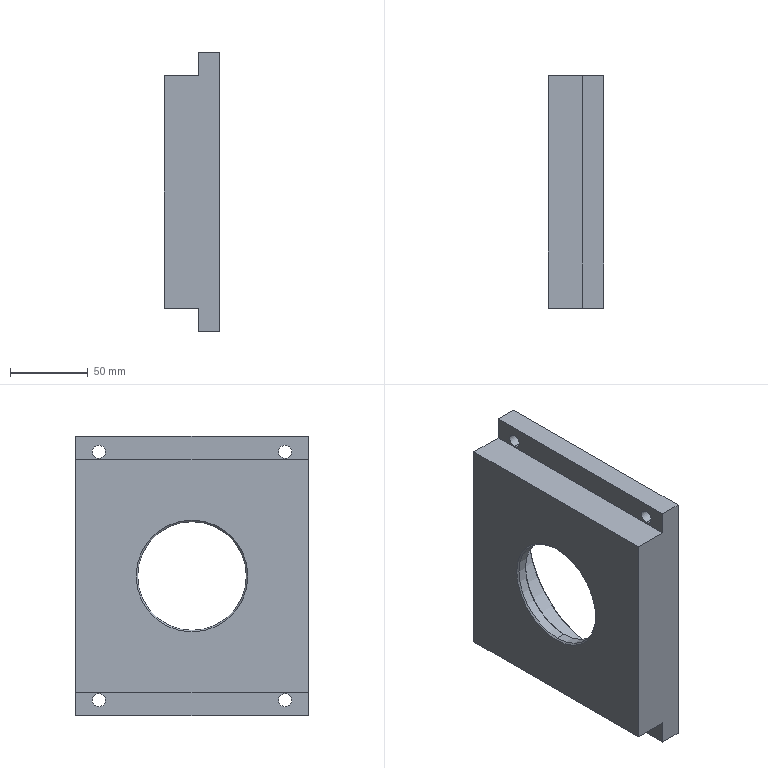Part | SolidWorks | features BaseBody 1 | 1 solid | 42 faces | box 36 x 150 x 180 mm | volume 519040 mm3 | cylinder 18 | cone 12 | plane 12 | commonest cylinder face diameters 8.5 x8 30.5 x4 70 x2 110 x2 120 x2
STEP:
#1=CARTESIAN_POINT('',(17.,0.,60.));
#2=VERTEX_POINT('',#1);
#3=CARTESIAN_POINT('',(17.,0.,-60.));
#4=VERTEX_POINT('',#3);
#5=CARTESIAN_POINT('',(17.,0.,0.));
#6=DIRECTION('',(1.,0.,0.));
#7=DIRECTION('',(0.,0.,-1.));
#8=AXIS2_PLACEMENT_3D('',#5,#6,#7);
#9=CIRCLE('',#8,60.);
#10=EDGE_CURVE('',#2,#4,#9,.T.);
#11=ORIENTED_EDGE('',*,*,#10,.F.);
#12=CARTESIAN_POINT('',(18.,0.,61.));
#13=VERTEX_POINT('',#12);
#14=CARTESIAN_POINT('',(17.,0.,60.));
#15=DIRECTION('',(0.7071,0.,0.7071));
#16=VECTOR('',#15,1000.);
#17=LINE('',#14,#16);
#18=EDGE_CURVE('',#2,#13,#17,.T.);
#19=ORIENTED_EDGE('',*,*,#18,.T.);
#20=CARTESIAN_POINT('',(18.,0.,-61.));
#21=VERTEX_POINT('',#20);
#22=CARTESIAN_POINT('',(18.,0.,0.));
#23=DIRECTION('',(-1.,0.,0.));
#24=DIRECTION('',(0.,0.,-1.));
#25=AXIS2_PLACEMENT_3D('',#22,#23,#24);
#26=CIRCLE('',#25,61.);
#27=EDGE_CURVE('',#21,#13,#26,.T.);
#28=ORIENTED_EDGE('',*,*,#27,.F.);
#29=CARTESIAN_POINT('',(17.,0.,-60.));
#30=DIRECTION('',(0.7071,0.,-0.7071));
#31=VECTOR('',#30,1000.);
#32=LINE('',#29,#31);
#33=EDGE_CURVE('',#4,#21,#32,.T.);
#34=ORIENTED_EDGE('',*,*,#33,.F.);
#35=EDGE_LOOP('',(#11,#19,#28,#34));
#36=FACE_OUTER_BOUND('',#35,.T.);
#37=CARTESIAN_POINT('',(17.,0.,0.));
#38=DIRECTION('',(1.,0.,0.));
#39=DIRECTION('',(0.,0.,-1.));
#40=AXIS2_PLACEMENT_3D('',#37,#38,#39);
#41=CONICAL_SURFACE('',#40,60.,0.7854);
#42=ADVANCED_FACE('',(#36),#41,.F.);
#43=CARTESIAN_POINT('',(-11.,0.,35.));
#44=VERTEX_POINT('',#43);
#45=CARTESIAN_POINT('',(-11.,0.,-35.));
#46=VERTEX_POINT('',#45);
#47=CARTESIAN_POINT('',(-11.,0.,0.));
#48=DIRECTION('',(1.,0.,0.));
#49=DIRECTION('',(0.,0.,-1.));
#50=AXIS2_PLACEMENT_3D('',#47,#48,#49);
#51=CIRCLE('',#50,35.);
#52=EDGE_CURVE('',#44,#46,#51,.T.);
#53=ORIENTED_EDGE('',*,*,#52,.F.);
#54=CARTESIAN_POINT('',(-10.,0.,36.));
#55=VERTEX_POINT('',#54);
#56=CARTESIAN_POINT('',(-11.,0.,35.));
#57=DIRECTION('',(0.7071,0.,0.7071));
#58=VECTOR('',#57,1000.);
#59=LINE('',#56,#58);
#60=EDGE_CURVE('',#44,#55,#59,.T.);
#61=ORIENTED_EDGE('',*,*,#60,.T.);
#62=CARTESIAN_POINT('',(-10.,0.,-36.));
#63=VERTEX_POINT('',#62);
#64=CARTESIAN_POINT('',(-10.,0.,0.));
#65=DIRECTION('',(-1.,0.,0.));
#66=DIRECTION('',(0.,0.,-1.));
#67=AXIS2_PLACEMENT_3D('',#64,#65,#66);
#68=CIRCLE('',#67,36.);
#69=EDGE_CURVE('',#63,#55,#68,.T.);
#70=ORIENTED_EDGE('',*,*,#69,.F.);
#71=CARTESIAN_POINT('',(-11.,0.,-35.));
#72=DIRECTION('',(0.7071,0.,-0.7071));
#73=VECTOR('',#72,1000.);
#74=LINE('',#71,#73);
#75=EDGE_CURVE('',#46,#63,#74,.T.);
#76=ORIENTED_EDGE('',*,*,#75,.F.);
#77=EDGE_LOOP('',(#53,#61,#70,#76));
#78=FACE_OUTER_BOUND('',#77,.T.);
#79=CARTESIAN_POINT('',(-11.,0.,0.));
#80=DIRECTION('',(1.,0.,0.));
#81=DIRECTION('',(0.,0.,-1.));
#82=AXIS2_PLACEMENT_3D('',#79,#80,#81);
#83=CONICAL_SURFACE('',#82,35.,0.7854);
#84=ADVANCED_FACE('',(#78),#83,.F.);
#85=CARTESIAN_POINT('',(-17.,0.,-35.));
#86=VERTEX_POINT('',#85);
#87=CARTESIAN_POINT('',(-17.,0.,35.));
#88=VERTEX_POINT('',#87);
#89=CARTESIAN_POINT('',(-17.,0.,0.));
#90=DIRECTION('',(-1.,0.,0.));
#91=DIRECTION('',(0.,0.,-1.));
#92=AXIS2_PLACEMENT_3D('',#89,#90,#91);
#93=CIRCLE('',#92,35.);
#94=EDGE_CURVE('',#86,#88,#93,.T.);
#95=ORIENTED_EDGE('',*,*,#94,.F.);
#96=CARTESIAN_POINT('',(-18.,0.,-36.));
#97=VERTEX_POINT('',#96);
#98=CARTESIAN_POINT('',(-18.,0.,-36.));
#99=DIRECTION('',(-0.7071,0.,-0.7071));
#100=VECTOR('',#99,1000.);
#101=LINE('',#98,#100);
#102=EDGE_CURVE('',#86,#97,#101,.T.);
#103=ORIENTED_EDGE('',*,*,#102,.T.);
#104=CARTESIAN_POINT('',(-18.,0.,36.));
#105=VERTEX_POINT('',#104);
#106=CARTESIAN_POINT('',(-18.,0.,0.));
#107=DIRECTION('',(1.,0.,0.));
#108=DIRECTION('',(0.,0.,-1.));
#109=AXIS2_PLACEMENT_3D('',#106,#107,#108);
#110=CIRCLE('',#109,36.);
#111=EDGE_CURVE('',#105,#97,#110,.T.);
#112=ORIENTED_EDGE('',*,*,#111,.F.);
#113=CARTESIAN_POINT('',(-18.,0.,36.));
#114=DIRECTION('',(-0.7071,0.,0.7071));
#115=VECTOR('',#114,1000.);
#116=LINE('',#113,#115);
#117=EDGE_CURVE('',#88,#105,#116,.T.);
#118=ORIENTED_EDGE('',*,*,#117,.F.);
#119=EDGE_LOOP('',(#95,#103,#112,#118));
#120=FACE_OUTER_BOUND('',#119,.T.);
#121=CARTESIAN_POINT('',(-18.,0.,0.));
#122=DIRECTION('',(-1.,0.,0.));
#123=DIRECTION('',(0.,0.,1.));
#124=AXIS2_PLACEMENT_3D('',#121,#122,#123);
#125=CONICAL_SURFACE('',#124,36.,0.7854);
#126=ADVANCED_FACE('',(#120),#125,.F.);
#127=CARTESIAN_POINT('',(-6.,0.,55.));
#128=VERTEX_POINT('',#127);
#129=CARTESIAN_POINT('',(-6.,0.,-55.));
#130=VERTEX_POINT('',#129);
#131=CARTESIAN_POINT('',(-6.,0.,0.));
#132=DIRECTION('',(1.,0.,0.));
#133=DIRECTION('',(0.,0.,-1.));
#134=AXIS2_PLACEMENT_3D('',#131,#132,#133);
#135=CIRCLE('',#134,55.);
#136=EDGE_CURVE('',#128,#130,#135,.T.);
#137=ORIENTED_EDGE('',*,*,#136,.F.);
#138=CARTESIAN_POINT('',(-5.,0.,56.));
#139=VERTEX_POINT('',#138);
#140=CARTESIAN_POINT('',(-6.,0.,55.));
#141=DIRECTION('',(0.7071,0.,0.7071));
#142=VECTOR('',#141,1000.);
#143=LINE('',#140,#142);
#144=EDGE_CURVE('',#128,#139,#143,.T.);
#145=ORIENTED_EDGE('',*,*,#144,.T.);
#146=CARTESIAN_POINT('',(-5.,0.,-56.));
#147=VERTEX_POINT('',#146);
#148=CARTESIAN_POINT('',(-5.,0.,0.));
#149=DIRECTION('',(-1.,0.,0.));
#150=DIRECTION('',(0.,0.,-1.));
#151=AXIS2_PLACEMENT_3D('',#148,#149,#150);
#152=CIRCLE('',#151,56.);
#153=EDGE_CURVE('',#147,#139,#152,.T.);
#154=ORIENTED_EDGE('',*,*,#153,.F.);
#155=CARTESIAN_POINT('',(-6.,0.,-55.));
#156=DIRECTION('',(0.7071,0.,-0.7071));
#157=VECTOR('',#156,1000.);
#158=LINE('',#155,#157);
#159=EDGE_CURVE('',#130,#147,#158,.T.);
#160=ORIENTED_EDGE('',*,*,#159,.F.);
#161=EDGE_LOOP('',(#137,#145,#154,#160));
#162=FACE_OUTER_BOUND('',#161,.T.);
#163=CARTESIAN_POINT('',(-6.,0.,0.));
#164=DIRECTION('',(1.,0.,0.));
#165=DIRECTION('',(0.,0.,-1.));
#166=AXIS2_PLACEMENT_3D('',#163,#164,#165);
#167=CONICAL_SURFACE('',#166,55.,0.7854);
#168=ADVANCED_FACE('',(#162),#167,.F.);
#169=CARTESIAN_POINT('',(0.,70.,-60.25));
#170=VERTEX_POINT('',#169);
#171=CARTESIAN_POINT('',(0.,70.,-29.75));
#172=VERTEX_POINT('',#171);
#173=CARTESIAN_POINT('',(0.,70.,-45.));
#174=DIRECTION('',(0.,1.,0.));
#175=DIRECTION('',(0.,0.,1.));
#176=AXIS2_PLACEMENT_3D('',#173,#174,#175);
#177=CIRCLE('',#176,15.25);
#178=EDGE_CURVE('',#170,#172,#177,.T.);
#179=ORIENTED_EDGE('',*,*,#178,.F.);
#180=CARTESIAN_POINT('',(0.,75.,-60.25));
#181=VERTEX_POINT('',#180);
#182=CARTESIAN_POINT('',(0.,75.,-60.25));
#183=DIRECTION('',(0.,1.,0.));
#184=VECTOR('',#183,1000.);
#185=LINE('',#182,#184);
#186=EDGE_CURVE('',#170,#181,#185,.T.);
#187=ORIENTED_EDGE('',*,*,#186,.T.);
#188=CARTESIAN_POINT('',(0.,75.,-29.75));
#189=VERTEX_POINT('',#188);
#190=CARTESIAN_POINT('',(0.,75.,-45.));
#191=DIRECTION('',(0.,1.,0.));
#192=DIRECTION('',(0.,0.,1.));
#193=AXIS2_PLACEMENT_3D('',#190,#191,#192);
#194=CIRCLE('',#193,15.25);
#195=EDGE_CURVE('',#181,#189,#194,.T.);
#196=ORIENTED_EDGE('',*,*,#195,.T.);
#197=CARTESIAN_POINT('',(0.,75.,-29.75));
#198=DIRECTION('',(0.,1.,0.));
#199=VECTOR('',#198,1000.);
#200=LINE('',#197,#199);
#201=EDGE_CURVE('',#172,#189,#200,.T.);
#202=ORIENTED_EDGE('',*,*,#201,.F.);
#203=EDGE_LOOP('',(#179,#187,#196,#202));
#204=FACE_OUTER_BOUND('',#203,.T.);
#205=CARTESIAN_POINT('',(0.,75.,-45.));
#206=DIRECTION('',(0.,1.,0.));
#207=DIRECTION('',(0.,0.,1.));
#208=AXIS2_PLACEMENT_3D('',#205,#206,#207);
#209=CYLINDRICAL_SURFACE('',#208,15.25);
#210=ADVANCED_FACE('',(#204),#209,.F.);
#211=CARTESIAN_POINT('',(0.,60.837,-45.));
#212=VERTEX_POINT('',#211);
#213=CARTESIAN_POINT('',(0.,70.,-29.75));
#214=DIRECTION('',(0.,0.515,0.8572));
#215=VECTOR('',#214,1000.);
#216=LINE('',#213,#215);
#217=EDGE_CURVE('',#212,#172,#216,.T.);
#218=ORIENTED_EDGE('',*,*,#217,.F.);
#219=CARTESIAN_POINT('',(0.,70.,-60.25));
#220=DIRECTION('',(0.,0.515,-0.8572));
#221=VECTOR('',#220,1000.);
#222=LINE('',#219,#221);
#223=EDGE_CURVE('',#212,#170,#222,.T.);
#224=ORIENTED_EDGE('',*,*,#223,.T.);
#225=ORIENTED_EDGE('',*,*,#178,.T.);
#226=EDGE_LOOP('',(#218,#224,#225));
#227=FACE_OUTER_BOUND('',#226,.T.);
#228=CARTESIAN_POINT('',(0.,70.,-45.));
#229=DIRECTION('',(0.,1.,0.));
#230=DIRECTION('',(0.,0.,1.));
#231=AXIS2_PLACEMENT_3D('',#228,#229,#230);
#232=CONICAL_SURFACE('',#231,15.25,1.03);
#233=ADVANCED_FACE('',(#227),#232,.F.);
#234=CARTESIAN_POINT('',(0.,70.,29.75));
#235=VERTEX_POINT('',#234);
#236=CARTESIAN_POINT('',(0.,70.,60.25));
#237=VERTEX_POINT('',#236);
#238=CARTESIAN_POINT('',(0.,70.,45.));
#239=DIRECTION('',(0.,1.,0.));
#240=DIRECTION('',(0.,0.,1.));
#241=AXIS2_PLACEMENT_3D('',#238,#239,#240);
#242=CIRCLE('',#241,15.25);
#243=EDGE_CURVE('',#235,#237,#242,.T.);
#244=ORIENTED_EDGE('',*,*,#243,.F.);
#245=CARTESIAN_POINT('',(0.,75.,29.75));
#246=VERTEX_POINT('',#245);
#247=CARTESIAN_POINT('',(0.,75.,29.75));
#248=DIRECTION('',(0.,1.,0.));
#249=VECTOR('',#248,1000.);
#250=LINE('',#247,#249);
#251=EDGE_CURVE('',#235,#246,#250,.T.);
#252=ORIENTED_EDGE('',*,*,#251,.T.);
#253=CARTESIAN_POINT('',(0.,75.,60.25));
#254=VERTEX_POINT('',#253);
#255=CARTESIAN_POINT('',(0.,75.,45.));
#256=DIRECTION('',(0.,1.,0.));
#257=DIRECTION('',(0.,0.,1.));
#258=AXIS2_PLACEMENT_3D('',#255,#256,#257);
#259=CIRCLE('',#258,15.25);
#260=EDGE_CURVE('',#246,#254,#259,.T.);
#261=ORIENTED_EDGE('',*,*,#260,.T.);
#262=CARTESIAN_POINT('',(0.,75.,60.25));
#263=DIRECTION('',(0.,1.,0.));
#264=VECTOR('',#263,1000.);
#265=LINE('',#262,#264);
#266=EDGE_CURVE('',#237,#254,#265,.T.);
#267=ORIENTED_EDGE('',*,*,#266,.F.);
#268=EDGE_LOOP('',(#244,#252,#261,#267));
#269=FACE_OUTER_BOUND('',#268,.T.);
#270=CARTESIAN_POINT('',(0.,75.,45.));
#271=DIRECTION('',(0.,1.,0.));
#272=DIRECTION('',(0.,0.,1.));
#273=AXIS2_PLACEMENT_3D('',#270,#271,#272);
#274=CYLINDRICAL_SURFACE('',#273,15.25);
#275=ADVANCED_FACE('',(#269),#274,.F.);
#276=CARTESIAN_POINT('',(0.,60.837,45.));
#277=VERTEX_POINT('',#276);
#278=CARTESIAN_POINT('',(0.,70.,60.25));
#279=DIRECTION('',(0.,0.515,0.8572));
#280=VECTOR('',#279,1000.);
#281=LINE('',#278,#280);
#282=EDGE_CURVE('',#277,#237,#281,.T.);
#283=ORIENTED_EDGE('',*,*,#282,.F.);
#284=CARTESIAN_POINT('',(0.,70.,29.75));
#285=DIRECTION('',(0.,0.515,-0.8572));
#286=VECTOR('',#285,1000.);
#287=LINE('',#284,#286);
#288=EDGE_CURVE('',#277,#235,#287,.T.);
#289=ORIENTED_EDGE('',*,*,#288,.T.);
#290=ORIENTED_EDGE('',*,*,#243,.T.);
#291=EDGE_LOOP('',(#283,#289,#290));
#292=FACE_OUTER_BOUND('',#291,.T.);
#293=CARTESIAN_POINT('',(0.,70.,45.));
#294=DIRECTION('',(0.,1.,0.));
#295=DIRECTION('',(0.,0.,1.));
#296=AXIS2_PLACEMENT_3D('',#293,#294,#295);
#297=CONICAL_SURFACE('',#296,15.25,1.03);
#298=ADVANCED_FACE('',(#292),#297,.F.);
#299=CARTESIAN_POINT('',(4.,60.,84.25));
#300=VERTEX_POINT('',#299);
#301=CARTESIAN_POINT('',(4.,60.,75.75));
#302=VERTEX_POINT('',#301);
#303=CARTESIAN_POINT('',(4.,60.,80.));
#304=DIRECTION('',(1.,0.,0.));
#305=DIRECTION('',(0.,0.,-1.));
#306=AXIS2_PLACEMENT_3D('',#303,#304,#305);
#307=CIRCLE('',#306,4.25);
#308=EDGE_CURVE('',#300,#302,#307,.T.);
#309=ORIENTED_EDGE('',*,*,#308,.F.);
#310=CARTESIAN_POINT('',(18.,60.,84.25));
#311=VERTEX_POINT('',#310);
#312=CARTESIAN_POINT('',(18.,60.,84.25));
#313=DIRECTION('',(1.,0.,0.));
#314=VECTOR('',#313,1000.);
#315=LINE('',#312,#314);
#316=EDGE_CURVE('',#300,#311,#315,.T.);
#317=ORIENTED_EDGE('',*,*,#316,.T.);
#318=CARTESIAN_POINT('',(18.,60.,75.75));
#319=VERTEX_POINT('',#318);
#320=CARTESIAN_POINT('',(18.,60.,80.));
#321=DIRECTION('',(1.,0.,0.));
#322=DIRECTION('',(0.,0.,-1.));
#323=AXIS2_PLACEMENT_3D('',#320,#321,#322);
#324=CIRCLE('',#323,4.25);
#325=EDGE_CURVE('',#311,#319,#324,.T.);
#326=ORIENTED_EDGE('',*,*,#325,.T.);
#327=CARTESIAN_POINT('',(18.,60.,75.75));
#328=DIRECTION('',(1.,0.,0.));
#329=VECTOR('',#328,1000.);
#330=LINE('',#327,#329);
#331=EDGE_CURVE('',#302,#319,#330,.T.);
#332=ORIENTED_EDGE('',*,*,#331,.F.);
#333=EDGE_LOOP('',(#309,#317,#326,#332));
#334=FACE_OUTER_BOUND('',#333,.T.);
#335=CARTESIAN_POINT('',(18.,60.,80.));
#336=DIRECTION('',(1.,0.,0.));
#337=DIRECTION('',(0.,0.,-1.));
#338=AXIS2_PLACEMENT_3D('',#335,#336,#337);
#339=CYLINDRICAL_SURFACE('',#338,4.25);
#340=ADVANCED_FACE('',(#334),#339,.F.);
#341=CARTESIAN_POINT('',(4.,60.,-75.75));
#342=VERTEX_POINT('',#341);
#343=CARTESIAN_POINT('',(4.,60.,-84.25));
#344=VERTEX_POINT('',#343);
#345=CARTESIAN_POINT('',(4.,60.,-80.));
#346=DIRECTION('',(1.,0.,0.));
#347=DIRECTION('',(0.,0.,-1.));
#348=AXIS2_PLACEMENT_3D('',#345,#346,#347);
#349=CIRCLE('',#348,4.25);
#350=EDGE_CURVE('',#342,#344,#349,.T.);
#351=ORIENTED_EDGE('',*,*,#350,.F.);
#352=CARTESIAN_POINT('',(18.,60.,-75.75));
#353=VERTEX_POINT('',#352);
#354=CARTESIAN_POINT('',(18.,60.,-75.75));
#355=DIRECTION('',(1.,0.,0.));
#356=VECTOR('',#355,1000.);
#357=LINE('',#354,#356);
#358=EDGE_CURVE('',#342,#353,#357,.T.);
#359=ORIENTED_EDGE('',*,*,#358,.T.);
#360=CARTESIAN_POINT('',(18.,60.,-84.25));
#361=VERTEX_POINT('',#360);
#362=CARTESIAN_POINT('',(18.,60.,-80.));
#363=DIRECTION('',(1.,0.,0.));
#364=DIRECTION('',(0.,0.,-1.));
#365=AXIS2_PLACEMENT_3D('',#362,#363,#364);
#366=CIRCLE('',#365,4.25);
#367=EDGE_CURVE('',#353,#361,#366,.T.);
#368=ORIENTED_EDGE('',*,*,#367,.T.);
#369=CARTESIAN_POINT('',(18.,60.,-84.25));
#370=DIRECTION('',(1.,0.,0.));
#371=VECTOR('',#370,1000.);
#372=LINE('',#369,#371);
#373=EDGE_CURVE('',#344,#361,#372,.T.);
#374=ORIENTED_EDGE('',*,*,#373,.F.);
#375=EDGE_LOOP('',(#351,#359,#368,#374));
#376=FACE_OUTER_BOUND('',#375,.T.);
#377=CARTESIAN_POINT('',(18.,60.,-80.));
#378=DIRECTION('',(1.,0.,0.));
#379=DIRECTION('',(0.,0.,-1.));
#380=AXIS2_PLACEMENT_3D('',#377,#378,#379);
#381=CYLINDRICAL_SURFACE('',#380,4.25);
#382=ADVANCED_FACE('',(#376),#381,.F.);
#383=CARTESIAN_POINT('',(4.,-60.,-75.75));
#384=VERTEX_POINT('',#383);
#385=CARTESIAN_POINT('',(4.,-60.,-84.25));
#386=VERTEX_POINT('',#385);
#387=CARTESIAN_POINT('',(4.,-60.,-80.));
#388=DIRECTION('',(1.,0.,0.));
#389=DIRECTION('',(0.,0.,-1.));
#390=AXIS2_PLACEMENT_3D('',#387,#388,#389);
#391=CIRCLE('',#390,4.25);
#392=EDGE_CURVE('',#384,#386,#391,.T.);
#393=ORIENTED_EDGE('',*,*,#392,.F.);
#394=CARTESIAN_POINT('',(18.,-60.,-75.75));
#395=VERTEX_POINT('',#394);
#396=CARTESIAN_POINT('',(18.,-60.,-75.75));
#397=DIRECTION('',(1.,0.,0.));
#398=VECTOR('',#397,1000.);
#399=LINE('',#396,#398);
#400=EDGE_CURVE('',#384,#395,#399,.T.);
#401=ORIENTED_EDGE('',*,*,#400,.T.);
#402=CARTESIAN_POINT('',(18.,-60.,-84.25));
#403=VERTEX_POINT('',#402);
#404=CARTESIAN_POINT('',(18.,-60.,-80.));
#405=DIRECTION('',(1.,0.,0.));
#406=DIRECTION('',(0.,0.,-1.));
#407=AXIS2_PLACEMENT_3D('',#404,#405,#406);
#408=CIRCLE('',#407,4.25);
#409=EDGE_CURVE('',#395,#403,#408,.T.);
#410=ORIENTED_EDGE('',*,*,#409,.T.);
#411=CARTESIAN_POINT('',(18.,-60.,-84.25));
#412=DIRECTION('',(1.,0.,0.));
#413=VECTOR('',#412,1000.);
#414=LINE('',#411,#413);
#415=EDGE_CURVE('',#386,#403,#414,.T.);
#416=ORIENTED_EDGE('',*,*,#415,.F.);
#417=EDGE_LOOP('',(#393,#401,#410,#416));
#418=FACE_OUTER_BOUND('',#417,.T.);
#419=CARTESIAN_POINT('',(18.,-60.,-80.));
#420=DIRECTION('',(1.,0.,0.));
#421=DIRECTION('',(0.,0.,-1.));
#422=AXIS2_PLACEMENT_3D('',#419,#420,#421);
#423=CYLINDRICAL_SURFACE('',#422,4.25);
#424=ADVANCED_FACE('',(#418),#423,.F.);
#425=CARTESIAN_POINT('',(4.,-60.,84.25));
#426=VERTEX_POINT('',#425);
#427=CARTESIAN_POINT('',(4.,-60.,75.75));
#428=VERTEX_POINT('',#427);
#429=CARTESIAN_POINT('',(4.,-60.,80.));
#430=DIRECTION('',(1.,0.,0.));
#431=DIRECTION('',(0.,0.,-1.));
#432=AXIS2_PLACEMENT_3D('',#429,#430,#431);
#433=CIRCLE('',#432,4.25);
#434=EDGE_CURVE('',#426,#428,#433,.T.);
#435=ORIENTED_EDGE('',*,*,#434,.F.);
#436=CARTESIAN_POINT('',(18.,-60.,84.25));
#437=VERTEX_POINT('',#436);
#438=CARTESIAN_POINT('',(18.,-60.,84.25));
#439=DIRECTION('',(1.,0.,0.));
#440=VECTOR('',#439,1000.);
#441=LINE('',#438,#440);
#442=EDGE_CURVE('',#426,#437,#441,.T.);
#443=ORIENTED_EDGE('',*,*,#442,.T.);
#444=CARTESIAN_POINT('',(18.,-60.,75.75));
#445=VERTEX_POINT('',#444);
#446=CARTESIAN_POINT('',(18.,-60.,80.));
#447=DIRECTION('',(1.,0.,0.));
#448=DIRECTION('',(0.,0.,-1.));
#449=AXIS2_PLACEMENT_3D('',#446,#447,#448);
#450=CIRCLE('',#449,4.25);
#451=EDGE_CURVE('',#437,#445,#450,.T.);
#452=ORIENTED_EDGE('',*,*,#451,.T.);
#453=CARTESIAN_POINT('',(18.,-60.,75.75));
#454=DIRECTION('',(1.,0.,0.));
#455=VECTOR('',#454,1000.);
#456=LINE('',#453,#455);
#457=EDGE_CURVE('',#428,#445,#456,.T.);
#458=ORIENTED_EDGE('',*,*,#457,.F.);
#459=EDGE_LOOP('',(#435,#443,#452,#458));
#460=FACE_OUTER_BOUND('',#459,.T.);
#461=CARTESIAN_POINT('',(18.,-60.,80.));
#462=DIRECTION('',(1.,0.,0.));
#463=DIRECTION('',(0.,0.,-1.));
#464=AXIS2_PLACEMENT_3D('',#461,#462,#463);
#465=CYLINDRICAL_SURFACE('',#464,4.25);
#466=ADVANCED_FACE('',(#460),#465,.F.);
#467=CARTESIAN_POINT('',(-10.,0.,55.));
#468=VERTEX_POINT('',#467);
#469=CARTESIAN_POINT('',(-10.,0.,-55.));
#470=VERTEX_POINT('',#469);
#471=CARTESIAN_POINT('',(-10.,0.,0.));
#472=DIRECTION('',(1.,0.,0.));
#473=DIRECTION('',(0.,0.,-1.));
#474=AXIS2_PLACEMENT_3D('',#471,#472,#473);
#475=CIRCLE('',#474,55.);
#476=EDGE_CURVE('',#468,#470,#475,.T.);
#477=ORIENTED_EDGE('',*,*,#476,.F.);
#478=CARTESIAN_POINT('',(-10.,0.,55.));
#479=DIRECTION('',(1.,0.,0.));
#480=VECTOR('',#479,1000.);
#481=LINE('',#478,#480);
#482=EDGE_CURVE('',#468,#128,#481,.T.);
#483=ORIENTED_EDGE('',*,*,#482,.T.);
#484=ORIENTED_EDGE('',*,*,#136,.T.);
#485=CARTESIAN_POINT('',(-10.,0.,-55.));
#486=DIRECTION('',(1.,0.,0.));
#487=VECTOR('',#486,1000.);
#488=LINE('',#485,#487);
#489=EDGE_CURVE('',#470,#130,#488,.T.);
#490=ORIENTED_EDGE('',*,*,#489,.F.);
#491=EDGE_LOOP('',(#477,#483,#484,#490));
#492=FACE_OUTER_BOUND('',#491,.T.);
#493=CARTESIAN_POINT('',(-10.,0.,0.));
#494=DIRECTION('',(1.,0.,0.));
#495=DIRECTION('',(0.,0.,-1.));
#496=AXIS2_PLACEMENT_3D('',#493,#494,#495);
#497=CYLINDRICAL_SURFACE('',#496,55.);
#498=ADVANCED_FACE('',(#492),#497,.F.);
#499=CARTESIAN_POINT('',(-5.,0.,60.));
#500=VERTEX_POINT('',#499);
#501=CARTESIAN_POINT('',(-5.,0.,-60.));
#502=VERTEX_POINT('',#501);
#503=CARTESIAN_POINT('',(-5.,0.,0.));
#504=DIRECTION('',(1.,0.,0.));
#505=DIRECTION('',(0.,0.,-1.));
#506=AXIS2_PLACEMENT_3D('',#503,#504,#505);
#507=CIRCLE('',#506,60.);
#508=EDGE_CURVE('',#500,#502,#507,.T.);
#509=ORIENTED_EDGE('',*,*,#508,.F.);
#510=CARTESIAN_POINT('',(-5.,0.,60.));
#511=DIRECTION('',(1.,0.,0.));
#512=VECTOR('',#511,1000.);
#513=LINE('',#510,#512);
#514=EDGE_CURVE('',#500,#2,#513,.T.);
#515=ORIENTED_EDGE('',*,*,#514,.T.);
#516=ORIENTED_EDGE('',*,*,#10,.T.);
#517=CARTESIAN_POINT('',(-5.,0.,-60.));
#518=DIRECTION('',(1.,0.,0.));
#519=VECTOR('',#518,1000.);
#520=LINE('',#517,#519);
#521=EDGE_CURVE('',#502,#4,#520,.T.);
#522=ORIENTED_EDGE('',*,*,#521,.F.);
#523=EDGE_LOOP('',(#509,#515,#516,#522));
#524=FACE_OUTER_BOUND('',#523,.T.);
#525=CARTESIAN_POINT('',(-5.,0.,0.));
#526=DIRECTION('',(1.,0.,0.));
#527=DIRECTION('',(0.,0.,-1.));
#528=AXIS2_PLACEMENT_3D('',#525,#526,#527);
#529=CYLINDRICAL_SURFACE('',#528,60.);
#530=ADVANCED_FACE('',(#524),#529,.F.);
#531=ORIENTED_EDGE('',*,*,#52,.T.);
#532=CARTESIAN_POINT('',(18.,0.,-35.));
#533=DIRECTION('',(-1.,0.,0.));
#534=VECTOR('',#533,1000.);
#535=LINE('',#532,#534);
#536=EDGE_CURVE('',#46,#86,#535,.T.);
#537=ORIENTED_EDGE('',*,*,#536,.T.);
#538=ORIENTED_EDGE('',*,*,#94,.T.);
#539=CARTESIAN_POINT('',(18.,0.,35.));
#540=DIRECTION('',(-1.,0.,0.));
#541=VECTOR('',#540,1000.);
#542=LINE('',#539,#541);
#543=EDGE_CURVE('',#44,#88,#542,.T.);
#544=ORIENTED_EDGE('',*,*,#543,.F.);
#545=EDGE_LOOP('',(#531,#537,#538,#544));
#546=FACE_OUTER_BOUND('',#545,.T.);
#547=CARTESIAN_POINT('',(18.,0.,0.));
#548=DIRECTION('',(-1.,0.,0.));
#549=DIRECTION('',(0.,0.,1.));
#550=AXIS2_PLACEMENT_3D('',#547,#548,#549);
#551=CYLINDRICAL_SURFACE('',#550,35.);
#552=ADVANCED_FACE('',(#546),#551,.F.);
#553=ORIENTED_EDGE('',*,*,#536,.F.);
#554=CARTESIAN_POINT('',(-11.,0.,0.));
#555=DIRECTION('',(1.,0.,0.));
#556=DIRECTION('',(0.,0.,-1.));
#557=AXIS2_PLACEMENT_3D('',#554,#555,#556);
#558=CIRCLE('',#557,35.);
#559=EDGE_CURVE('',#46,#44,#558,.T.);
#560=ORIENTED_EDGE('',*,*,#559,.T.);
#561=ORIENTED_EDGE('',*,*,#543,.T.);
#562=CARTESIAN_POINT('',(-17.,0.,0.));
#563=DIRECTION('',(-1.,0.,0.));
#564=DIRECTION('',(0.,0.,-1.));
#565=AXIS2_PLACEMENT_3D('',#562,#563,#564);
#566=CIRCLE('',#565,35.);
#567=EDGE_CURVE('',#88,#86,#566,.T.);
#568=ORIENTED_EDGE('',*,*,#567,.T.);
#569=EDGE_LOOP('',(#553,#560,#561,#568));
#570=FACE_OUTER_BOUND('',#569,.T.);
#571=CARTESIAN_POINT('',(18.,0.,0.));
#572=DIRECTION('',(-1.,0.,0.));
#573=DIRECTION('',(0.,0.,1.));
#574=AXIS2_PLACEMENT_3D('',#571,#572,#573);
#575=CYLINDRICAL_SURFACE('',#574,35.);
#576=ADVANCED_FACE('',(#570),#575,.F.);
#577=ORIENTED_EDGE('',*,*,#27,.T.);
#578=CARTESIAN_POINT('',(18.,0.,0.));
#579=DIRECTION('',(-1.,0.,0.));
#580=DIRECTION('',(0.,0.,-1.));
#581=AXIS2_PLACEMENT_3D('',#578,#579,#580);
#582=CIRCLE('',#581,61.);
#583=EDGE_CURVE('',#13,#21,#582,.T.);
#584=ORIENTED_EDGE('',*,*,#583,.T.);
#585=EDGE_LOOP('',(#577,#584));
#586=FACE_BOUND('',#585,.T.);
#587=CARTESIAN_POINT('',(18.,60.,80.));
#588=DIRECTION('',(1.,0.,0.));
#589=DIRECTION('',(0.,0.,-1.));
#590=AXIS2_PLACEMENT_3D('',#587,#588,#589);
#591=CIRCLE('',#590,4.25);
#592=EDGE_CURVE('',#319,#311,#591,.T.);
#593=ORIENTED_EDGE('',*,*,#592,.F.);
#594=ORIENTED_EDGE('',*,*,#325,.F.);
#595=EDGE_LOOP('',(#593,#594));
#596=FACE_BOUND('',#595,.T.);
#597=CARTESIAN_POINT('',(18.,60.,-80.));
#598=DIRECTION('',(1.,0.,0.));
#599=DIRECTION('',(0.,0.,-1.));
#600=AXIS2_PLACEMENT_3D('',#597,#598,#599);
#601=CIRCLE('',#600,4.25);
#602=EDGE_CURVE('',#361,#353,#601,.T.);
#603=ORIENTED_EDGE('',*,*,#602,.F.);
#604=ORIENTED_EDGE('',*,*,#367,.F.);
#605=EDGE_LOOP('',(#603,#604));
#606=FACE_BOUND('',#605,.T.);
#607=CARTESIAN_POINT('',(18.,-60.,-80.));
#608=DIRECTION('',(1.,0.,0.));
#609=DIRECTION('',(0.,0.,-1.));
#610=AXIS2_PLACEMENT_3D('',#607,#608,#609);
#611=CIRCLE('',#610,4.25);
#612=EDGE_CURVE('',#403,#395,#611,.T.);
#613=ORIENTED_EDGE('',*,*,#612,.F.);
#614=ORIENTED_EDGE('',*,*,#409,.F.);
#615=EDGE_LOOP('',(#613,#614));
#616=FACE_BOUND('',#615,.T.);
#617=CARTESIAN_POINT('',(18.,-60.,80.));
#618=DIRECTION('',(1.,0.,0.));
#619=DIRECTION('',(0.,0.,-1.));
#620=AXIS2_PLACEMENT_3D('',#617,#618,#619);
#621=CIRCLE('',#620,4.25);
#622=EDGE_CURVE('',#445,#437,#621,.T.);
#623=ORIENTED_EDGE('',*,*,#622,.F.);
#624=ORIENTED_EDGE('',*,*,#451,.F.);
#625=EDGE_LOOP('',(#623,#624));
#626=FACE_BOUND('',#625,.T.);
#627=CARTESIAN_POINT('',(18.,-75.,-90.));
#628=VERTEX_POINT('',#627);
#629=CARTESIAN_POINT('',(18.,75.,-90.));
#630=VERTEX_POINT('',#629);
#631=CARTESIAN_POINT('',(18.,75.,-90.));
#632=DIRECTION('',(0.,1.,0.));
#633=VECTOR('',#632,1000.);
#634=LINE('',#631,#633);
#635=EDGE_CURVE('',#628,#630,#634,.T.);
#636=ORIENTED_EDGE('',*,*,#635,.T.);
#637=CARTESIAN_POINT('',(18.,75.,90.));
#638=VERTEX_POINT('',#637);
#639=CARTESIAN_POINT('',(18.,75.,90.));
#640=DIRECTION('',(0.,0.,1.));
#641=VECTOR('',#640,1000.);
#642=LINE('',#639,#641);
#643=EDGE_CURVE('',#630,#638,#642,.T.);
#644=ORIENTED_EDGE('',*,*,#643,.T.);
#645=CARTESIAN_POINT('',(18.,-75.,90.));
#646=VERTEX_POINT('',#645);
#647=CARTESIAN_POINT('',(18.,75.,90.));
#648=DIRECTION('',(0.,-1.,0.));
#649=VECTOR('',#648,1000.);
#650=LINE('',#647,#649);
#651=EDGE_CURVE('',#638,#646,#650,.T.);
#652=ORIENTED_EDGE('',*,*,#651,.T.);
#653=CARTESIAN_POINT('',(18.,-75.,90.));
#654=DIRECTION('',(0.,0.,-1.));
#655=VECTOR('',#654,1000.);
#656=LINE('',#653,#655);
#657=EDGE_CURVE('',#646,#628,#656,.T.);
#658=ORIENTED_EDGE('',*,*,#657,.T.);
#659=EDGE_LOOP('',(#636,#644,#652,#658));
#660=FACE_OUTER_BOUND('',#659,.T.);
#661=CARTESIAN_POINT('',(18.,0.,0.));
#662=DIRECTION('',(1.,0.,0.));
#663=DIRECTION('',(0.,0.,-1.));
#664=AXIS2_PLACEMENT_3D('',#661,#662,#663);
#665=PLANE('',#664);
#666=ADVANCED_FACE('',(#586,#596,#606,#616,#626,#660),#665,.T.);
#667=ORIENTED_EDGE('',*,*,#111,.T.);
#668=CARTESIAN_POINT('',(-18.,0.,0.));
#669=DIRECTION('',(1.,0.,0.));
#670=DIRECTION('',(0.,0.,-1.));
#671=AXIS2_PLACEMENT_3D('',#668,#669,#670);
#672=CIRCLE('',#671,36.);
#673=EDGE_CURVE('',#97,#105,#672,.T.);
#674=ORIENTED_EDGE('',*,*,#673,.T.);
#675=EDGE_LOOP('',(#667,#674));
#676=FACE_BOUND('',#675,.T.);
#677=CARTESIAN_POINT('',(-18.,75.,-75.));
#678=VERTEX_POINT('',#677);
#679=CARTESIAN_POINT('',(-18.,75.,75.));
#680=VERTEX_POINT('',#679);
#681=CARTESIAN_POINT('',(-18.,75.,90.));
#682=DIRECTION('',(0.,0.,1.));
#683=VECTOR('',#682,1000.);
#684=LINE('',#681,#683);
#685=EDGE_CURVE('',#678,#680,#684,.T.);
#686=ORIENTED_EDGE('',*,*,#685,.F.);
#687=CARTESIAN_POINT('',(-18.,-75.,-75.));
#688=VERTEX_POINT('',#687);
#689=CARTESIAN_POINT('',(-18.,-75.,-75.));
#690=DIRECTION('',(0.,1.,0.));
#691=VECTOR('',#690,1000.);
#692=LINE('',#689,#691);
#693=EDGE_CURVE('',#688,#678,#692,.T.);
#694=ORIENTED_EDGE('',*,*,#693,.F.);
#695=CARTESIAN_POINT('',(-18.,-75.,75.));
#696=VERTEX_POINT('',#695);
#697=CARTESIAN_POINT('',(-18.,-75.,90.));
#698=DIRECTION('',(0.,0.,-1.));
#699=VECTOR('',#698,1000.);
#700=LINE('',#697,#699);
#701=EDGE_CURVE('',#696,#688,#700,.T.);
#702=ORIENTED_EDGE('',*,*,#701,.F.);
#703=CARTESIAN_POINT('',(-18.,-75.,75.));
#704=DIRECTION('',(0.,1.,0.));
#705=VECTOR('',#704,1000.);
#706=LINE('',#703,#705);
#707=EDGE_CURVE('',#696,#680,#706,.T.);
#708=ORIENTED_EDGE('',*,*,#707,.T.);
#709=EDGE_LOOP('',(#686,#694,#702,#708));
#710=FACE_OUTER_BOUND('',#709,.T.);
#711=CARTESIAN_POINT('',(-18.,0.,0.));
#712=DIRECTION('',(1.,0.,0.));
#713=DIRECTION('',(0.,0.,-1.));
#714=AXIS2_PLACEMENT_3D('',#711,#712,#713);
#715=PLANE('',#714);
#716=ADVANCED_FACE('',(#676,#710),#715,.F.);
#717=CARTESIAN_POINT('',(4.,-75.,-90.));
#718=VERTEX_POINT('',#717);
#719=CARTESIAN_POINT('',(18.,-75.,-90.));
#720=DIRECTION('',(-1.,0.,0.));
#721=VECTOR('',#720,1000.);
#722=LINE('',#719,#721);
#723=EDGE_CURVE('',#628,#718,#722,.T.);
#724=ORIENTED_EDGE('',*,*,#723,.T.);
#725=CARTESIAN_POINT('',(4.,75.,-90.));
#726=VERTEX_POINT('',#725);
#727=CARTESIAN_POINT('',(4.,-75.,-90.));
#728=DIRECTION('',(0.,1.,0.));
#729=VECTOR('',#728,1000.);
#730=LINE('',#727,#729);
#731=EDGE_CURVE('',#718,#726,#730,.T.);
#732=ORIENTED_EDGE('',*,*,#731,.T.);
#733=CARTESIAN_POINT('',(18.,75.,-90.));
#734=DIRECTION('',(-1.,0.,0.));
#735=VECTOR('',#734,1000.);
#736=LINE('',#733,#735);
#737=EDGE_CURVE('',#630,#726,#736,.T.);
#738=ORIENTED_EDGE('',*,*,#737,.F.);
#739=ORIENTED_EDGE('',*,*,#635,.F.);
#740=EDGE_LOOP('',(#724,#732,#738,#739));
#741=FACE_OUTER_BOUND('',#740,.T.);
#742=CARTESIAN_POINT('',(18.,75.,-90.));
#743=DIRECTION('',(0.,0.,1.));
#744=DIRECTION('',(1.,0.,0.));
#745=AXIS2_PLACEMENT_3D('',#742,#743,#744);
#746=PLANE('',#745);
#747=ADVANCED_FACE('',(#741),#746,.F.);
#748=CARTESIAN_POINT('',(0.,75.,-45.));
#749=DIRECTION('',(0.,1.,0.));
#750=DIRECTION('',(0.,0.,1.));
#751=AXIS2_PLACEMENT_3D('',#748,#749,#750);
#752=CIRCLE('',#751,15.25);
#753=EDGE_CURVE('',#189,#181,#752,.T.);
#754=ORIENTED_EDGE('',*,*,#753,.F.);
#755=ORIENTED_EDGE('',*,*,#195,.F.);
#756=EDGE_LOOP('',(#754,#755));
#757=FACE_BOUND('',#756,.T.);
#758=CARTESIAN_POINT('',(0.,75.,45.));
#759=DIRECTION('',(0.,1.,0.));
#760=DIRECTION('',(0.,0.,1.));
#761=AXIS2_PLACEMENT_3D('',#758,#759,#760);
#762=CIRCLE('',#761,15.25);
#763=EDGE_CURVE('',#254,#246,#762,.T.);
#764=ORIENTED_EDGE('',*,*,#763,.F.);
#765=ORIENTED_EDGE('',*,*,#260,.F.);
#766=EDGE_LOOP('',(#764,#765));
#767=FACE_BOUND('',#766,.T.);
#768=ORIENTED_EDGE('',*,*,#737,.T.);
#769=CARTESIAN_POINT('',(4.,75.,-75.));
#770=VERTEX_POINT('',#769);
#771=CARTESIAN_POINT('',(4.,75.,-90.));
#772=DIRECTION('',(0.,0.,-1.));
#773=VECTOR('',#772,1000.);
#774=LINE('',#771,#773);
#775=EDGE_CURVE('',#770,#726,#774,.T.);
#776=ORIENTED_EDGE('',*,*,#775,.F.);
#777=CARTESIAN_POINT('',(-18.,75.,-75.));
#778=DIRECTION('',(1.,0.,0.));
#779=VECTOR('',#778,1000.);
#780=LINE('',#777,#779);
#781=EDGE_CURVE('',#678,#770,#780,.T.);
#782=ORIENTED_EDGE('',*,*,#781,.F.);
#783=ORIENTED_EDGE('',*,*,#685,.T.);
#784=CARTESIAN_POINT('',(4.,75.,75.));
#785=VERTEX_POINT('',#784);
#786=CARTESIAN_POINT('',(-18.,75.,75.));
#787=DIRECTION('',(-1.,0.,0.));
#788=VECTOR('',#787,1000.);
#789=LINE('',#786,#788);
#790=EDGE_CURVE('',#785,#680,#789,.T.);
#791=ORIENTED_EDGE('',*,*,#790,.F.);
#792=CARTESIAN_POINT('',(4.,75.,90.));
#793=VERTEX_POINT('',#792);
#794=CARTESIAN_POINT('',(4.,75.,90.));
#795=DIRECTION('',(0.,0.,-1.));
#796=VECTOR('',#795,1000.);
#797=LINE('',#794,#796);
#798=EDGE_CURVE('',#793,#785,#797,.T.);
#799=ORIENTED_EDGE('',*,*,#798,.F.);
#800=CARTESIAN_POINT('',(18.,75.,90.));
#801=DIRECTION('',(-1.,0.,0.));
#802=VECTOR('',#801,1000.);
#803=LINE('',#800,#802);
#804=EDGE_CURVE('',#638,#793,#803,.T.);
#805=ORIENTED_EDGE('',*,*,#804,.F.);
#806=ORIENTED_EDGE('',*,*,#643,.F.);
#807=EDGE_LOOP('',(#768,#776,#782,#783,#791,#799,#805,#806));
#808=FACE_OUTER_BOUND('',#807,.T.);
#809=CARTESIAN_POINT('',(18.,75.,90.));
#810=DIRECTION('',(0.,-1.,0.));
#811=DIRECTION('',(0.,0.,-1.));
#812=AXIS2_PLACEMENT_3D('',#809,#810,#811);
#813=PLANE('',#812);
#814=ADVANCED_FACE('',(#757,#767,#808),#813,.F.);
#815=ORIENTED_EDGE('',*,*,#804,.T.);
#816=CARTESIAN_POINT('',(4.,-75.,90.));
#817=VERTEX_POINT('',#816);
#818=CARTESIAN_POINT('',(4.,-75.,90.));
#819=DIRECTION('',(0.,1.,0.));
#820=VECTOR('',#819,1000.);
#821=LINE('',#818,#820);
#822=EDGE_CURVE('',#817,#793,#821,.T.);
#823=ORIENTED_EDGE('',*,*,#822,.F.);
#824=CARTESIAN_POINT('',(18.,-75.,90.));
#825=DIRECTION('',(-1.,0.,0.));
#826=VECTOR('',#825,1000.);
#827=LINE('',#824,#826);
#828=EDGE_CURVE('',#646,#817,#827,.T.);
#829=ORIENTED_EDGE('',*,*,#828,.F.);
#830=ORIENTED_EDGE('',*,*,#651,.F.);
#831=EDGE_LOOP('',(#815,#823,#829,#830));
#832=FACE_OUTER_BOUND('',#831,.T.);
#833=CARTESIAN_POINT('',(18.,75.,90.));
#834=DIRECTION('',(0.,0.,-1.));
#835=DIRECTION('',(-1.,0.,0.));
#836=AXIS2_PLACEMENT_3D('',#833,#834,#835);
#837=PLANE('',#836);
#838=ADVANCED_FACE('',(#832),#837,.F.);
#839=CARTESIAN_POINT('',(4.,-75.,-75.));
#840=VERTEX_POINT('',#839);
#841=CARTESIAN_POINT('',(-18.,-75.,-75.));
#842=DIRECTION('',(1.,0.,0.));
#843=VECTOR('',#842,1000.);
#844=LINE('',#841,#843);
#845=EDGE_CURVE('',#688,#840,#844,.T.);
#846=ORIENTED_EDGE('',*,*,#845,.T.);
#847=CARTESIAN_POINT('',(4.,-75.,-90.));
#848=DIRECTION('',(0.,0.,-1.));
#849=VECTOR('',#848,1000.);
#850=LINE('',#847,#849);
#851=EDGE_CURVE('',#840,#718,#850,.T.);
#852=ORIENTED_EDGE('',*,*,#851,.T.);
#853=ORIENTED_EDGE('',*,*,#723,.F.);
#854=ORIENTED_EDGE('',*,*,#657,.F.);
#855=ORIENTED_EDGE('',*,*,#828,.T.);
#856=CARTESIAN_POINT('',(4.,-75.,75.));
#857=VERTEX_POINT('',#856);
#858=CARTESIAN_POINT('',(4.,-75.,90.));
#859=DIRECTION('',(0.,0.,-1.));
#860=VECTOR('',#859,1000.);
#861=LINE('',#858,#860);
#862=EDGE_CURVE('',#817,#857,#861,.T.);
#863=ORIENTED_EDGE('',*,*,#862,.T.);
#864=CARTESIAN_POINT('',(-18.,-75.,75.));
#865=DIRECTION('',(-1.,0.,0.));
#866=VECTOR('',#865,1000.);
#867=LINE('',#864,#866);
#868=EDGE_CURVE('',#857,#696,#867,.T.);
#869=ORIENTED_EDGE('',*,*,#868,.T.);
#870=ORIENTED_EDGE('',*,*,#701,.T.);
#871=EDGE_LOOP('',(#846,#852,#853,#854,#855,#863,#869,#870));
#872=FACE_OUTER_BOUND('',#871,.T.);
#873=CARTESIAN_POINT('',(18.,-75.,90.));
#874=DIRECTION('',(0.,1.,0.));
#875=DIRECTION('',(0.,0.,1.));
#876=AXIS2_PLACEMENT_3D('',#873,#874,#875);
#877=PLANE('',#876);
#878=ADVANCED_FACE('',(#872),#877,.F.);
#879=ORIENTED_EDGE('',*,*,#514,.F.);
#880=CARTESIAN_POINT('',(-5.,0.,0.));
#881=DIRECTION('',(1.,0.,0.));
#882=DIRECTION('',(0.,0.,-1.));
#883=AXIS2_PLACEMENT_3D('',#880,#881,#882);
#884=CIRCLE('',#883,60.);
#885=EDGE_CURVE('',#502,#500,#884,.T.);
#886=ORIENTED_EDGE('',*,*,#885,.F.);
#887=ORIENTED_EDGE('',*,*,#521,.T.);
#888=CARTESIAN_POINT('',(17.,0.,0.));
#889=DIRECTION('',(1.,0.,0.));
#890=DIRECTION('',(0.,0.,-1.));
#891=AXIS2_PLACEMENT_3D('',#888,#889,#890);
#892=CIRCLE('',#891,60.);
#893=EDGE_CURVE('',#4,#2,#892,.T.);
#894=ORIENTED_EDGE('',*,*,#893,.T.);
#895=EDGE_LOOP('',(#879,#886,#887,#894));
#896=FACE_OUTER_BOUND('',#895,.T.);
#897=CARTESIAN_POINT('',(-5.,0.,0.));
#898=DIRECTION('',(1.,0.,0.));
#899=DIRECTION('',(0.,0.,-1.));
#900=AXIS2_PLACEMENT_3D('',#897,#898,#899);
#901=CYLINDRICAL_SURFACE('',#900,60.);
#902=ADVANCED_FACE('',(#896),#901,.F.);
#903=ORIENTED_EDGE('',*,*,#153,.T.);
#904=CARTESIAN_POINT('',(-5.,0.,0.));
#905=DIRECTION('',(-1.,0.,0.));
#906=DIRECTION('',(0.,0.,-1.));
#907=AXIS2_PLACEMENT_3D('',#904,#905,#906);
#908=CIRCLE('',#907,56.);
#909=EDGE_CURVE('',#139,#147,#908,.T.);
#910=ORIENTED_EDGE('',*,*,#909,.T.);
#911=EDGE_LOOP('',(#903,#910));
#912=FACE_BOUND('',#911,.T.);
#913=ORIENTED_EDGE('',*,*,#885,.T.);
#914=ORIENTED_EDGE('',*,*,#508,.T.);
#915=EDGE_LOOP('',(#913,#914));
#916=FACE_OUTER_BOUND('',#915,.T.);
#917=CARTESIAN_POINT('',(-5.,0.,0.));
#918=DIRECTION('',(1.,0.,0.));
#919=DIRECTION('',(0.,0.,-1.));
#920=AXIS2_PLACEMENT_3D('',#917,#918,#919);
#921=PLANE('',#920);
#922=ADVANCED_FACE('',(#912,#916),#921,.T.);
#923=ORIENTED_EDGE('',*,*,#482,.F.);
#924=CARTESIAN_POINT('',(-10.,0.,0.));
#925=DIRECTION('',(1.,0.,0.));
#926=DIRECTION('',(0.,0.,-1.));
#927=AXIS2_PLACEMENT_3D('',#924,#925,#926);
#928=CIRCLE('',#927,55.);
#929=EDGE_CURVE('',#470,#468,#928,.T.);
#930=ORIENTED_EDGE('',*,*,#929,.F.);
#931=ORIENTED_EDGE('',*,*,#489,.T.);
#932=CARTESIAN_POINT('',(-6.,0.,0.));
#933=DIRECTION('',(1.,0.,0.));
#934=DIRECTION('',(0.,0.,-1.));
#935=AXIS2_PLACEMENT_3D('',#932,#933,#934);
#936=CIRCLE('',#935,55.);
#937=EDGE_CURVE('',#130,#128,#936,.T.);
#938=ORIENTED_EDGE('',*,*,#937,.T.);
#939=EDGE_LOOP('',(#923,#930,#931,#938));
#940=FACE_OUTER_BOUND('',#939,.T.);
#941=CARTESIAN_POINT('',(-10.,0.,0.));
#942=DIRECTION('',(1.,0.,0.));
#943=DIRECTION('',(0.,0.,-1.));
#944=AXIS2_PLACEMENT_3D('',#941,#942,#943);
#945=CYLINDRICAL_SURFACE('',#944,55.);
#946=ADVANCED_FACE('',(#940),#945,.F.);
#947=ORIENTED_EDGE('',*,*,#69,.T.);
#948=CARTESIAN_POINT('',(-10.,0.,0.));
#949=DIRECTION('',(-1.,0.,0.));
#950=DIRECTION('',(0.,0.,-1.));
#951=AXIS2_PLACEMENT_3D('',#948,#949,#950);
#952=CIRCLE('',#951,36.);
#953=EDGE_CURVE('',#55,#63,#952,.T.);
#954=ORIENTED_EDGE('',*,*,#953,.T.);
#955=EDGE_LOOP('',(#947,#954));
#956=FACE_BOUND('',#955,.T.);
#957=ORIENTED_EDGE('',*,*,#929,.T.);
#958=ORIENTED_EDGE('',*,*,#476,.T.);
#959=EDGE_LOOP('',(#957,#958));
#960=FACE_OUTER_BOUND('',#959,.T.);
#961=CARTESIAN_POINT('',(-10.,0.,0.));
#962=DIRECTION('',(1.,0.,0.));
#963=DIRECTION('',(0.,0.,-1.));
#964=AXIS2_PLACEMENT_3D('',#961,#962,#963);
#965=PLANE('',#964);
#966=ADVANCED_FACE('',(#956,#960),#965,.T.);
#967=ORIENTED_EDGE('',*,*,#707,.F.);
#968=ORIENTED_EDGE('',*,*,#868,.F.);
#969=CARTESIAN_POINT('',(4.,-75.,75.));
#970=DIRECTION('',(0.,1.,0.));
#971=VECTOR('',#970,1000.);
#972=LINE('',#969,#971);
#973=EDGE_CURVE('',#857,#785,#972,.T.);
#974=ORIENTED_EDGE('',*,*,#973,.T.);
#975=ORIENTED_EDGE('',*,*,#790,.T.);
#976=EDGE_LOOP('',(#967,#968,#974,#975));
#977=FACE_OUTER_BOUND('',#976,.T.);
#978=CARTESIAN_POINT('',(-18.,-75.,75.));
#979=DIRECTION('',(0.,0.,-1.));
#980=DIRECTION('',(-1.,0.,0.));
#981=AXIS2_PLACEMENT_3D('',#978,#979,#980);
#982=PLANE('',#981);
#983=ADVANCED_FACE('',(#977),#982,.F.);
#984=CARTESIAN_POINT('',(4.,60.,80.));
#985=DIRECTION('',(1.,0.,0.));
#986=DIRECTION('',(0.,0.,-1.));
#987=AXIS2_PLACEMENT_3D('',#984,#985,#986);
#988=CIRCLE('',#987,4.25);
#989=EDGE_CURVE('',#302,#300,#988,.T.);
#990=ORIENTED_EDGE('',*,*,#989,.T.);
#991=ORIENTED_EDGE('',*,*,#308,.T.);
#992=EDGE_LOOP('',(#990,#991));
#993=FACE_BOUND('',#992,.T.);
#994=CARTESIAN_POINT('',(4.,-60.,80.));
#995=DIRECTION('',(1.,0.,0.));
#996=DIRECTION('',(0.,0.,-1.));
#997=AXIS2_PLACEMENT_3D('',#994,#995,#996);
#998=CIRCLE('',#997,4.25);
#999=EDGE_CURVE('',#428,#426,#998,.T.);
#1000=ORIENTED_EDGE('',*,*,#999,.T.);
#1001=ORIENTED_EDGE('',*,*,#434,.T.);
#1002=EDGE_LOOP('',(#1000,#1001));
#1003=FACE_BOUND('',#1002,.T.);
#1004=ORIENTED_EDGE('',*,*,#973,.F.);
#1005=ORIENTED_EDGE('',*,*,#862,.F.);
#1006=ORIENTED_EDGE('',*,*,#822,.T.);
#1007=ORIENTED_EDGE('',*,*,#798,.T.);
#1008=EDGE_LOOP('',(#1004,#1005,#1006,#1007));
#1009=FACE_OUTER_BOUND('',#1008,.T.);
#1010=CARTESIAN_POINT('',(4.,-75.,90.));
#1011=DIRECTION('',(1.,0.,0.));
#1012=DIRECTION('',(0.,0.,-1.));
#1013=AXIS2_PLACEMENT_3D('',#1010,#1011,#1012);
#1014=PLANE('',#1013);
#1015=ADVANCED_FACE('',(#993,#1003,#1009),#1014,.F.);
#1016=CARTESIAN_POINT('',(4.,60.,-80.));
#1017=DIRECTION('',(1.,0.,0.));
#1018=DIRECTION('',(0.,0.,-1.));
#1019=AXIS2_PLACEMENT_3D('',#1016,#1017,#1018);
#1020=CIRCLE('',#1019,4.25);
#1021=EDGE_CURVE('',#344,#342,#1020,.T.);
#1022=ORIENTED_EDGE('',*,*,#1021,.T.);
#1023=ORIENTED_EDGE('',*,*,#350,.T.);
#1024=EDGE_LOOP('',(#1022,#1023));
#1025=FACE_BOUND('',#1024,.T.);
#1026=CARTESIAN_POINT('',(4.,-60.,-80.));
#1027=DIRECTION('',(1.,0.,0.));
#1028=DIRECTION('',(0.,0.,-1.));
#1029=AXIS2_PLACEMENT_3D('',#1026,#1027,#1028);
#1030=CIRCLE('',#1029,4.25);
#1031=EDGE_CURVE('',#386,#384,#1030,.T.);
#1032=ORIENTED_EDGE('',*,*,#1031,.T.);
#1033=ORIENTED_EDGE('',*,*,#392,.T.);
#1034=EDGE_LOOP('',(#1032,#1033));
#1035=FACE_BOUND('',#1034,.T.);
#1036=ORIENTED_EDGE('',*,*,#731,.F.);
#1037=ORIENTED_EDGE('',*,*,#851,.F.);
#1038=CARTESIAN_POINT('',(4.,-75.,-75.));
#1039=DIRECTION('',(0.,1.,0.));
#1040=VECTOR('',#1039,1000.);
#1041=LINE('',#1038,#1040);
#1042=EDGE_CURVE('',#840,#770,#1041,.T.);
#1043=ORIENTED_EDGE('',*,*,#1042,.T.);
#1044=ORIENTED_EDGE('',*,*,#775,.T.);
#1045=EDGE_LOOP('',(#1036,#1037,#1043,#1044));
#1046=FACE_OUTER_BOUND('',#1045,.T.);
#1047=CARTESIAN_POINT('',(4.,-75.,-90.));
#1048=DIRECTION('',(1.,0.,0.));
#1049=DIRECTION('',(0.,0.,-1.));
#1050=AXIS2_PLACEMENT_3D('',#1047,#1048,#1049);
#1051=PLANE('',#1050);
#1052=ADVANCED_FACE('',(#1025,#1035,#1046),#1051,.F.);
#1053=ORIENTED_EDGE('',*,*,#1042,.F.);
#1054=ORIENTED_EDGE('',*,*,#845,.F.);
#1055=ORIENTED_EDGE('',*,*,#693,.T.);
#1056=ORIENTED_EDGE('',*,*,#781,.T.);
#1057=EDGE_LOOP('',(#1053,#1054,#1055,#1056));
#1058=FACE_OUTER_BOUND('',#1057,.T.);
#1059=CARTESIAN_POINT('',(-18.,-75.,-75.));
#1060=DIRECTION('',(0.,0.,1.));
#1061=DIRECTION('',(1.,0.,0.));
#1062=AXIS2_PLACEMENT_3D('',#1059,#1060,#1061);
#1063=PLANE('',#1062);
#1064=ADVANCED_FACE('',(#1058),#1063,.F.);
#1065=ORIENTED_EDGE('',*,*,#442,.F.);
#1066=ORIENTED_EDGE('',*,*,#999,.F.);
#1067=ORIENTED_EDGE('',*,*,#457,.T.);
#1068=ORIENTED_EDGE('',*,*,#622,.T.);
#1069=EDGE_LOOP('',(#1065,#1066,#1067,#1068));
#1070=FACE_OUTER_BOUND('',#1069,.T.);
#1071=CARTESIAN_POINT('',(18.,-60.,80.));
#1072=DIRECTION('',(1.,0.,0.));
#1073=DIRECTION('',(0.,0.,-1.));
#1074=AXIS2_PLACEMENT_3D('',#1071,#1072,#1073);
#1075=CYLINDRICAL_SURFACE('',#1074,4.25);
#1076=ADVANCED_FACE('',(#1070),#1075,.F.);
#1077=ORIENTED_EDGE('',*,*,#400,.F.);
#1078=ORIENTED_EDGE('',*,*,#1031,.F.);
#1079=ORIENTED_EDGE('',*,*,#415,.T.);
#1080=ORIENTED_EDGE('',*,*,#612,.T.);
#1081=EDGE_LOOP('',(#1077,#1078,#1079,#1080));
#1082=FACE_OUTER_BOUND('',#1081,.T.);
#1083=CARTESIAN_POINT('',(18.,-60.,-80.));
#1084=DIRECTION('',(1.,0.,0.));
#1085=DIRECTION('',(0.,0.,-1.));
#1086=AXIS2_PLACEMENT_3D('',#1083,#1084,#1085);
#1087=CYLINDRICAL_SURFACE('',#1086,4.25);
#1088=ADVANCED_FACE('',(#1082),#1087,.F.);
#1089=ORIENTED_EDGE('',*,*,#358,.F.);
#1090=ORIENTED_EDGE('',*,*,#1021,.F.);
#1091=ORIENTED_EDGE('',*,*,#373,.T.);
#1092=ORIENTED_EDGE('',*,*,#602,.T.);
#1093=EDGE_LOOP('',(#1089,#1090,#1091,#1092));
#1094=FACE_OUTER_BOUND('',#1093,.T.);
#1095=CARTESIAN_POINT('',(18.,60.,-80.));
#1096=DIRECTION('',(1.,0.,0.));
#1097=DIRECTION('',(0.,0.,-1.));
#1098=AXIS2_PLACEMENT_3D('',#1095,#1096,#1097);
#1099=CYLINDRICAL_SURFACE('',#1098,4.25);
#1100=ADVANCED_FACE('',(#1094),#1099,.F.);
#1101=ORIENTED_EDGE('',*,*,#316,.F.);
#1102=ORIENTED_EDGE('',*,*,#989,.F.);
#1103=ORIENTED_EDGE('',*,*,#331,.T.);
#1104=ORIENTED_EDGE('',*,*,#592,.T.);
#1105=EDGE_LOOP('',(#1101,#1102,#1103,#1104));
#1106=FACE_OUTER_BOUND('',#1105,.T.);
#1107=CARTESIAN_POINT('',(18.,60.,80.));
#1108=DIRECTION('',(1.,0.,0.));
#1109=DIRECTION('',(0.,0.,-1.));
#1110=AXIS2_PLACEMENT_3D('',#1107,#1108,#1109);
#1111=CYLINDRICAL_SURFACE('',#1110,4.25);
#1112=ADVANCED_FACE('',(#1106),#1111,.F.);
#1113=ORIENTED_EDGE('',*,*,#288,.F.);
#1114=ORIENTED_EDGE('',*,*,#282,.T.);
#1115=CARTESIAN_POINT('',(0.,70.,45.));
#1116=DIRECTION('',(0.,1.,0.));
#1117=DIRECTION('',(0.,0.,1.));
#1118=AXIS2_PLACEMENT_3D('',#1115,#1116,#1117);
#1119=CIRCLE('',#1118,15.25);
#1120=EDGE_CURVE('',#237,#235,#1119,.T.);
#1121=ORIENTED_EDGE('',*,*,#1120,.T.);
#1122=EDGE_LOOP('',(#1113,#1114,#1121));
#1123=FACE_OUTER_BOUND('',#1122,.T.);
#1124=CARTESIAN_POINT('',(0.,70.,45.));
#1125=DIRECTION('',(0.,1.,0.));
#1126=DIRECTION('',(0.,0.,1.));
#1127=AXIS2_PLACEMENT_3D('',#1124,#1125,#1126);
#1128=CONICAL_SURFACE('',#1127,15.25,1.03);
#1129=ADVANCED_FACE('',(#1123),#1128,.F.);
#1130=ORIENTED_EDGE('',*,*,#251,.F.);
#1131=ORIENTED_EDGE('',*,*,#1120,.F.);
#1132=ORIENTED_EDGE('',*,*,#266,.T.);
#1133=ORIENTED_EDGE('',*,*,#763,.T.);
#1134=EDGE_LOOP('',(#1130,#1131,#1132,#1133));
#1135=FACE_OUTER_BOUND('',#1134,.T.);
#1136=CARTESIAN_POINT('',(0.,75.,45.));
#1137=DIRECTION('',(0.,1.,0.));
#1138=DIRECTION('',(0.,0.,1.));
#1139=AXIS2_PLACEMENT_3D('',#1136,#1137,#1138);
#1140=CYLINDRICAL_SURFACE('',#1139,15.25);
#1141=ADVANCED_FACE('',(#1135),#1140,.F.);
#1142=ORIENTED_EDGE('',*,*,#223,.F.);
#1143=ORIENTED_EDGE('',*,*,#217,.T.);
#1144=CARTESIAN_POINT('',(0.,70.,-45.));
#1145=DIRECTION('',(0.,1.,0.));
#1146=DIRECTION('',(0.,0.,1.));
#1147=AXIS2_PLACEMENT_3D('',#1144,#1145,#1146);
#1148=CIRCLE('',#1147,15.25);
#1149=EDGE_CURVE('',#172,#170,#1148,.T.);
#1150=ORIENTED_EDGE('',*,*,#1149,.T.);
#1151=EDGE_LOOP('',(#1142,#1143,#1150));
#1152=FACE_OUTER_BOUND('',#1151,.T.);
#1153=CARTESIAN_POINT('',(0.,70.,-45.));
#1154=DIRECTION('',(0.,1.,0.));
#1155=DIRECTION('',(0.,0.,1.));
#1156=AXIS2_PLACEMENT_3D('',#1153,#1154,#1155);
#1157=CONICAL_SURFACE('',#1156,15.25,1.03);
#1158=ADVANCED_FACE('',(#1152),#1157,.F.);
#1159=ORIENTED_EDGE('',*,*,#186,.F.);
#1160=ORIENTED_EDGE('',*,*,#1149,.F.);
#1161=ORIENTED_EDGE('',*,*,#201,.T.);
#1162=ORIENTED_EDGE('',*,*,#753,.T.);
#1163=EDGE_LOOP('',(#1159,#1160,#1161,#1162));
#1164=FACE_OUTER_BOUND('',#1163,.T.);
#1165=CARTESIAN_POINT('',(0.,75.,-45.));
#1166=DIRECTION('',(0.,1.,0.));
#1167=DIRECTION('',(0.,0.,1.));
#1168=AXIS2_PLACEMENT_3D('',#1165,#1166,#1167);
#1169=CYLINDRICAL_SURFACE('',#1168,15.25);
#1170=ADVANCED_FACE('',(#1164),#1169,.F.);
#1171=ORIENTED_EDGE('',*,*,#144,.F.);
#1172=ORIENTED_EDGE('',*,*,#937,.F.);
#1173=ORIENTED_EDGE('',*,*,#159,.T.);
#1174=ORIENTED_EDGE('',*,*,#909,.F.);
#1175=EDGE_LOOP('',(#1171,#1172,#1173,#1174));
#1176=FACE_OUTER_BOUND('',#1175,.T.);
#1177=CARTESIAN_POINT('',(-6.,0.,0.));
#1178=DIRECTION('',(1.,0.,0.));
#1179=DIRECTION('',(0.,0.,-1.));
#1180=AXIS2_PLACEMENT_3D('',#1177,#1178,#1179);
#1181=CONICAL_SURFACE('',#1180,55.,0.7854);
#1182=ADVANCED_FACE('',(#1176),#1181,.F.);
#1183=ORIENTED_EDGE('',*,*,#102,.F.);
#1184=ORIENTED_EDGE('',*,*,#567,.F.);
#1185=ORIENTED_EDGE('',*,*,#117,.T.);
#1186=ORIENTED_EDGE('',*,*,#673,.F.);
#1187=EDGE_LOOP('',(#1183,#1184,#1185,#1186));
#1188=FACE_OUTER_BOUND('',#1187,.T.);
#1189=CARTESIAN_POINT('',(-18.,0.,0.));
#1190=DIRECTION('',(-1.,0.,0.));
#1191=DIRECTION('',(0.,0.,1.));
#1192=AXIS2_PLACEMENT_3D('',#1189,#1190,#1191);
#1193=CONICAL_SURFACE('',#1192,36.,0.7854);
#1194=ADVANCED_FACE('',(#1188),#1193,.F.);
#1195=ORIENTED_EDGE('',*,*,#60,.F.);
#1196=ORIENTED_EDGE('',*,*,#559,.F.);
#1197=ORIENTED_EDGE('',*,*,#75,.T.);
#1198=ORIENTED_EDGE('',*,*,#953,.F.);
#1199=EDGE_LOOP('',(#1195,#1196,#1197,#1198));
#1200=FACE_OUTER_BOUND('',#1199,.T.);
#1201=CARTESIAN_POINT('',(-11.,0.,0.));
#1202=DIRECTION('',(1.,0.,0.));
#1203=DIRECTION('',(0.,0.,-1.));
#1204=AXIS2_PLACEMENT_3D('',#1201,#1202,#1203);
#1205=CONICAL_SURFACE('',#1204,35.,0.7854);
#1206=ADVANCED_FACE('',(#1200),#1205,.F.);
#1207=ORIENTED_EDGE('',*,*,#18,.F.);
#1208=ORIENTED_EDGE('',*,*,#893,.F.);
#1209=ORIENTED_EDGE('',*,*,#33,.T.);
#1210=ORIENTED_EDGE('',*,*,#583,.F.);
#1211=EDGE_LOOP('',(#1207,#1208,#1209,#1210));
#1212=FACE_OUTER_BOUND('',#1211,.T.);
#1213=CARTESIAN_POINT('',(17.,0.,0.));
#1214=DIRECTION('',(1.,0.,0.));
#1215=DIRECTION('',(0.,0.,-1.));
#1216=AXIS2_PLACEMENT_3D('',#1213,#1214,#1215);
#1217=CONICAL_SURFACE('',#1216,60.,0.7854);
#1218=ADVANCED_FACE('',(#1212),#1217,.F.);
#1219=CLOSED_SHELL('',(#42,#84,#126,#168,#210,#233,#275,#298,#340,#382,#424,#466,#498,#530,#552,#576,#666,#716,#747,#814,#838,#878,#902,#922,#946,#966,#983,#1015,#1052,#1064,#1076,#1088,#1100,#1112,#1129,#1141,#1158,#1170,#1182,#1194,#1206,#1218));
#1220=MANIFOLD_SOLID_BREP('',#1219);
#1221=CARTESIAN_POINT('',(0.,0.,0.));
#1222=DIRECTION('',(0.,0.,1.));
#1223=DIRECTION('',(1.,0.,0.));
#1224=AXIS2_PLACEMENT_3D('',#1221,#1222,#1223);
#1225=(LENGTH_UNIT()NAMED_UNIT(*)SI_UNIT(.MILLI.,.METRE.));
#1226=UNCERTAINTY_MEASURE_WITH_UNIT(LENGTH_MEASURE(0.00001),#1225,'','');
#1227=(NAMED_UNIT(*)PLANE_ANGLE_UNIT()SI_UNIT($,.RADIAN.));
#1228=(NAMED_UNIT(*)SI_UNIT($,.STERADIAN.)SOLID_ANGLE_UNIT());
#1229=(GEOMETRIC_REPRESENTATION_CONTEXT(3)GLOBAL_UNCERTAINTY_ASSIGNED_CONTEXT((#1226))GLOBAL_UNIT_ASSIGNED_CONTEXT((#1225,#1227,#1228))REPRESENTATION_CONTEXT('',''));
#1230=ADVANCED_BREP_SHAPE_REPRESENTATION('',(#1220,#1224),#1229);